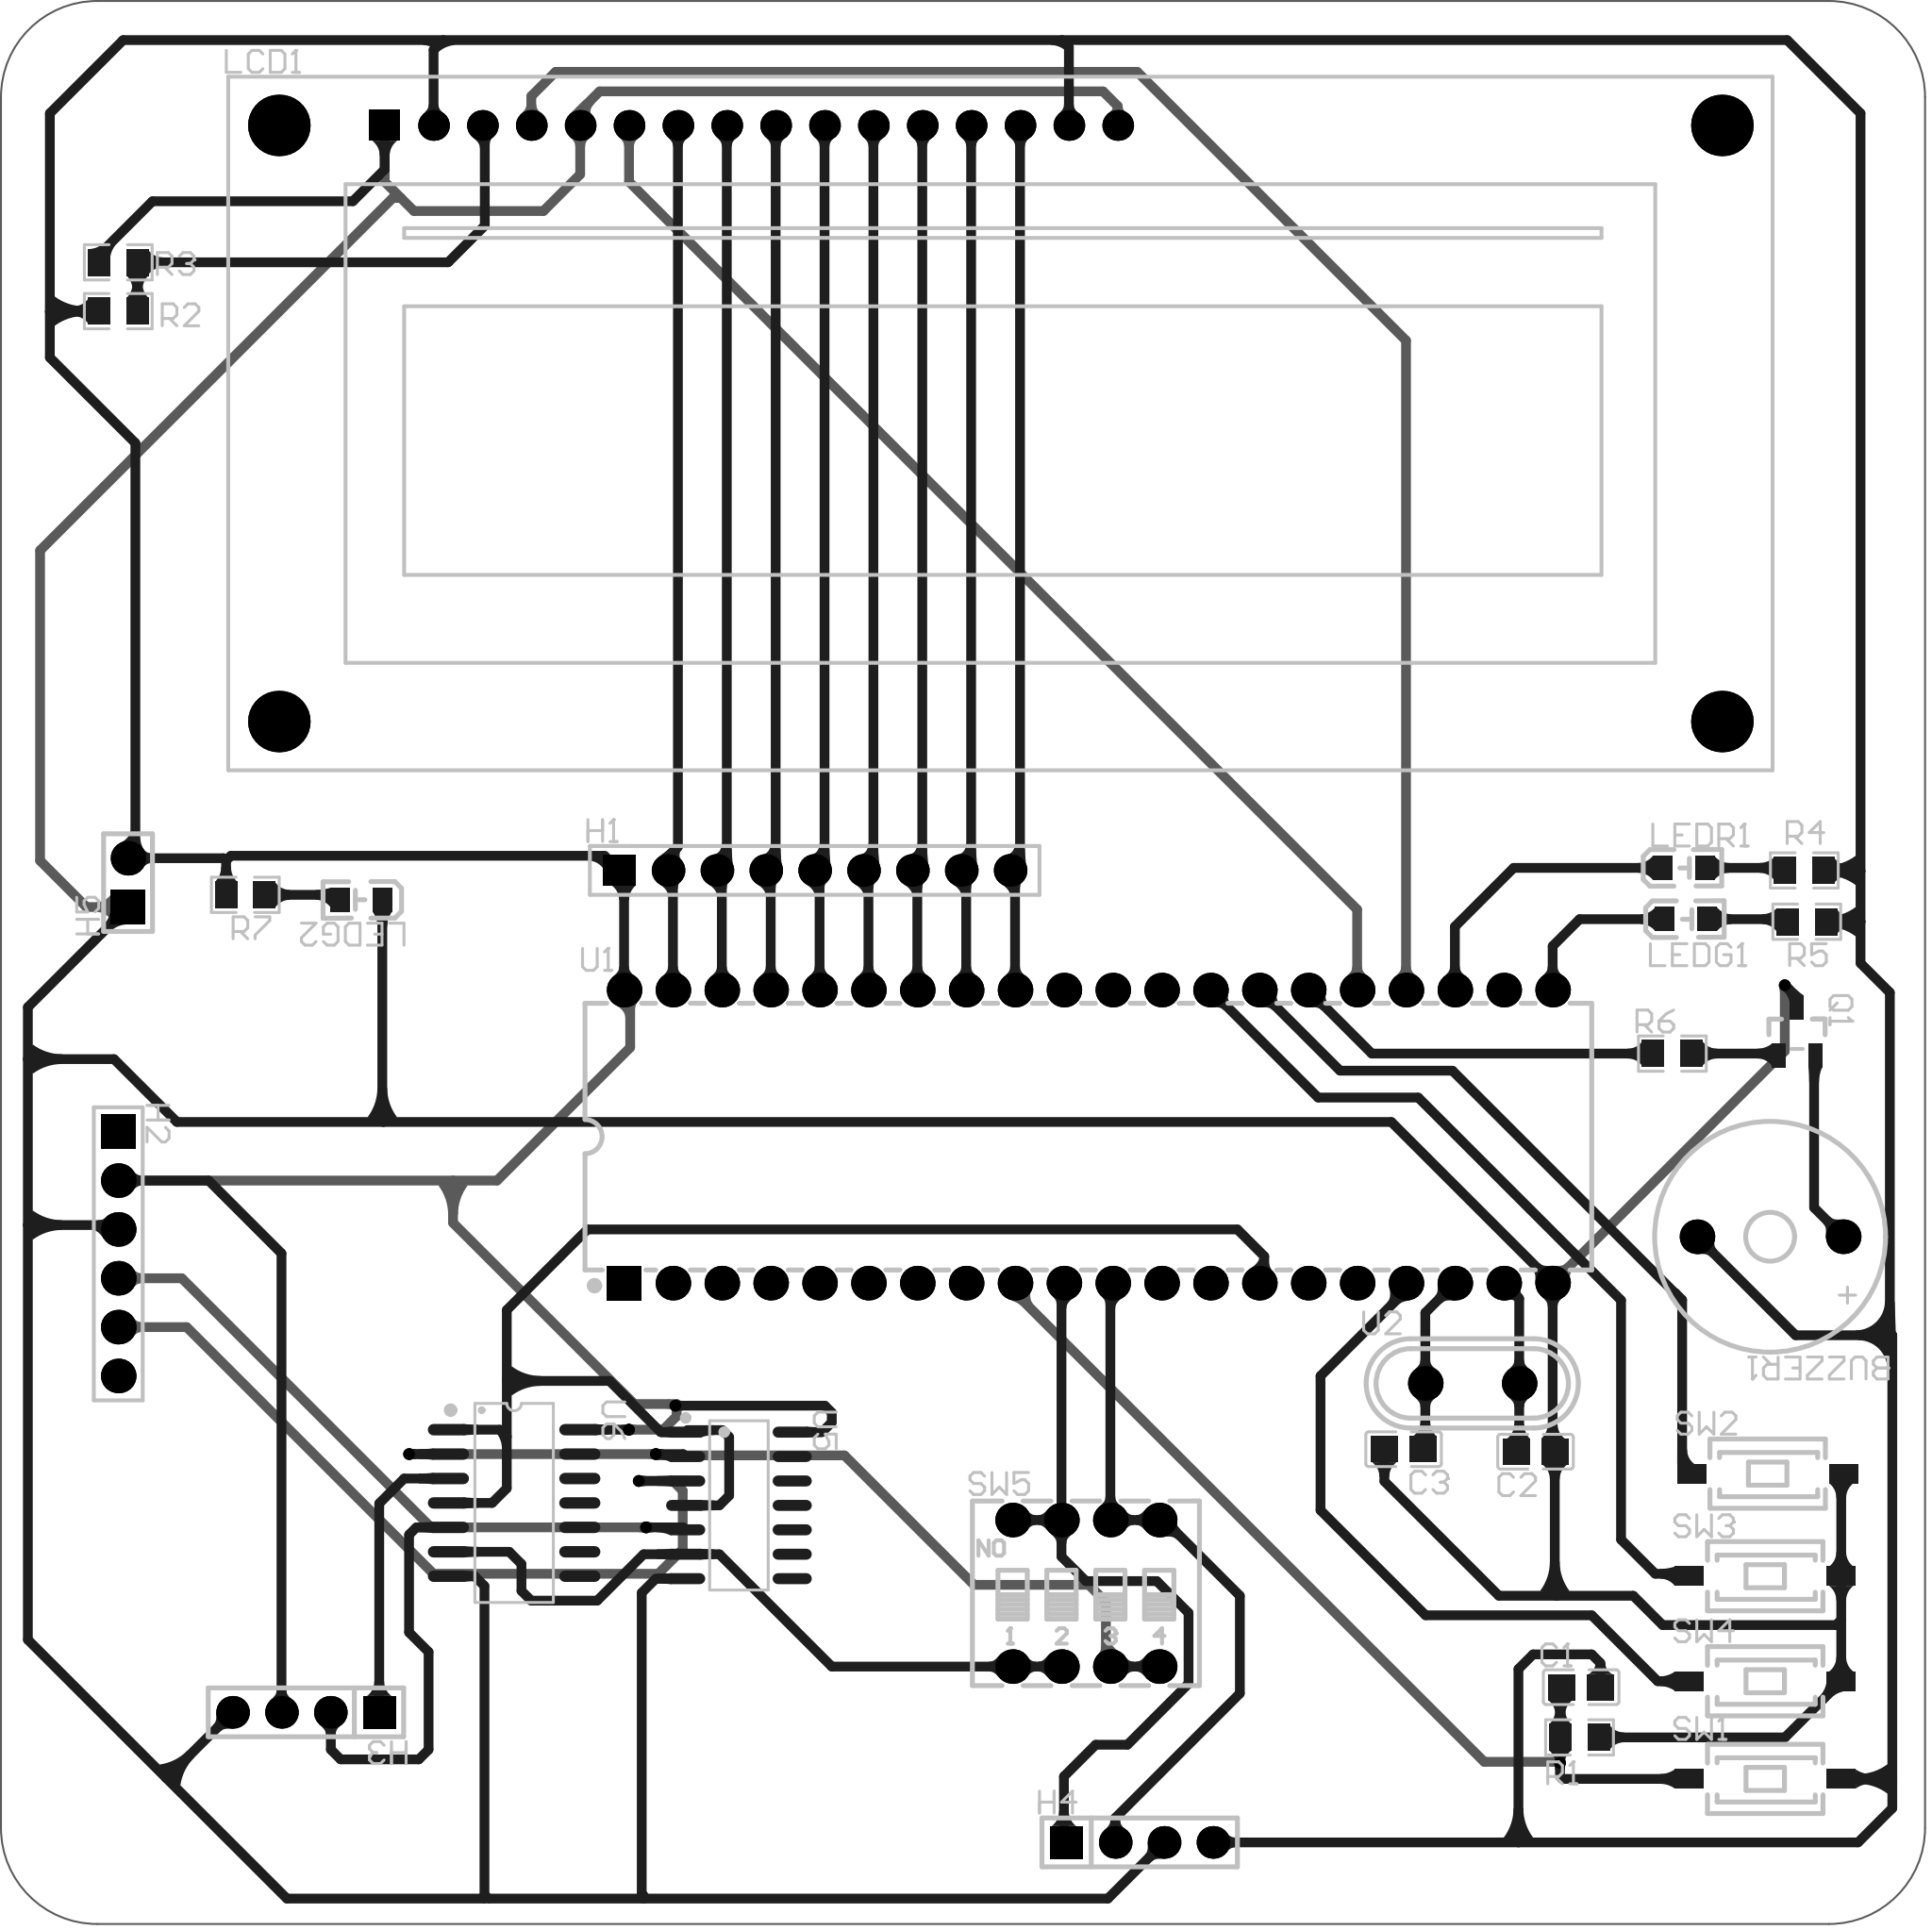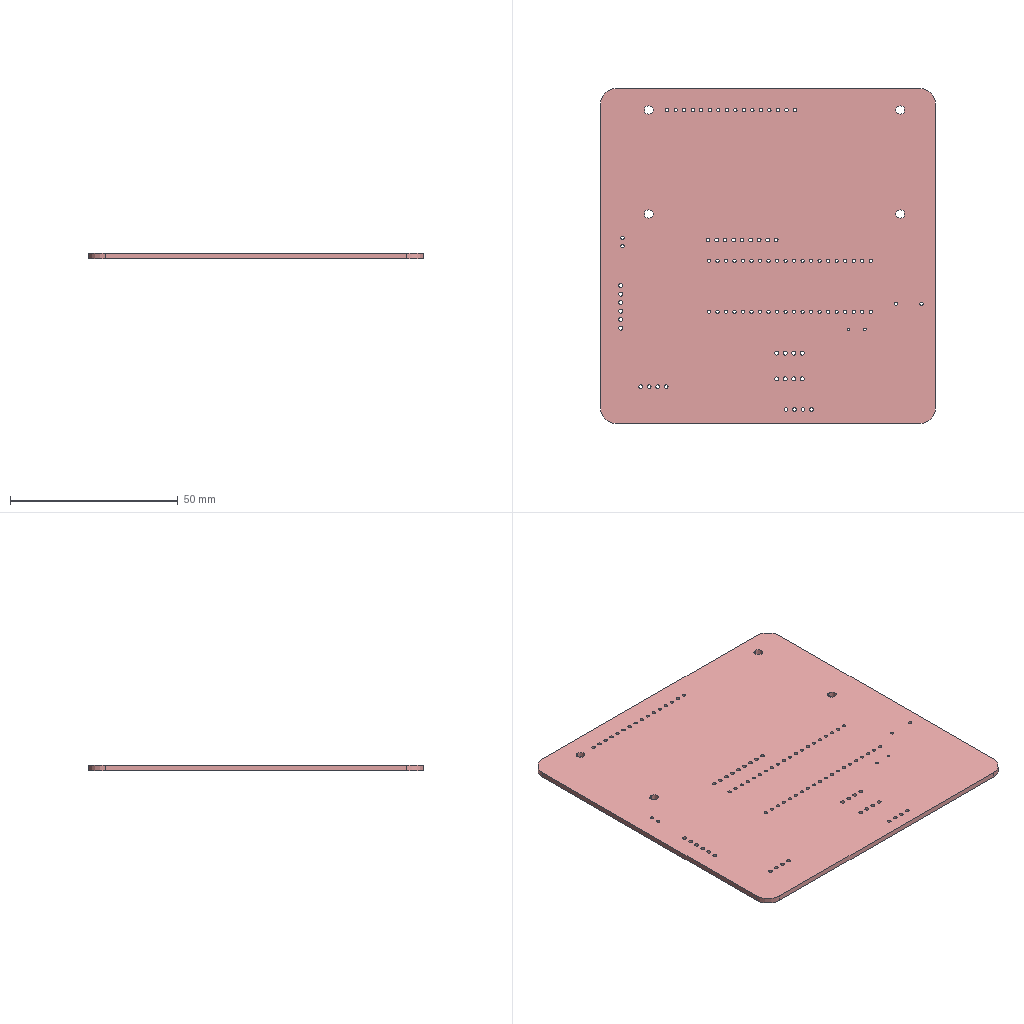Circuit board layout | Altium Designer | box 100 x 100 x 1.6 mm
Layer stack:
# Altium Designer layer stack of  (unit mm; dielectric type: 0 none, 1 core, 2 prepreg, 3 surface material)
index,name,kind,layer,copper_thickness_mm,dielectric_type,dielectric_thickness_mm,dielectric_material,dielectric_constant
0,Top Paste Mask Layer,other,,,,,,
1,Top Silkscreen Layer,other,,,,,,
2,Top Solder Mask Layer,dielectric,,,3,0.01,,3.3
3,Top Layer,copper,Top Layer,0.035,,,,
4,Dielectric1,dielectric,,,3,1.51,FR4,4.5
5,Bottom Layer,copper,Bottom Layer,0.035,,,,
6,Bottom Solder Mask Layer,dielectric,,,3,0.01,,3.3
7,Bottom Silkscreen Layer,other,,,,,,
8,Bottom Paste Mask Layer,other,,,,,,
# drill layer pairs: low layer,high layer
drill_pair,Top Layer,Bottom Layer
Part placement:
Designator,Comment,Layer,Footprint,Center-X(mm),Center-Y(mm),Rotation
BUZZER1,buzzer-12X9,TopLayer,BUZ-TH_BD12.0-P7.60-D0.6-FD,168.148,111.938,180
C1,10uf,TopLayer,C0805,158.327,88.516,0
C2,30pf,TopLayer,C0805,149.098,100.889,0
C3,30pf,TopLayer,C0805,155.956,100.762,180
H1,,TopLayer,HDR-TH_9P-P2.54-V-F-1,118.491,130.988,0
H2,,TopLayer,HDR-TH_6P-P2.54-V-M-1,82.296,111.049,270
H3,,TopLayer,HDR-TH_4P-P2.54-V-M,92.05,87.207,180
H4,,TopLayer,HDR-TH_4P-P2.54-V-M,135.382,80.442,0
LCD1,LMB162ADC,TopLayer,LCD1602,128.143,154.229,0
LEDG1,,TopLayer,LED_0805,163.78,128.453,0
LEDR1,,TopLayer,LED_0805,163.653,131.12,0
Q1,2N3906S-RTK/PS,TopLayer,SOT-23-3_L2.9-W1.3-P1.90-LS2.4-TR,169.545,122.606,270
R1,10K,TopLayer,R0805,158.242,85.903,0
R2,10K,TopLayer,R0805,82.296,160.071,180
R3,1K,TopLayer,R0805,82.296,162.611,0
R4,220,TopLayer,R0805,169.926,130.988,0
R5,220,TopLayer,R0805,170.053,128.321,0
R6,2.2K,TopLayer,R0805,163.068,121.463,0
SW5,DSWB04LHGET,TopLayer,SW-TH_DSWB04LHGET,132.588,93.396,0
U1,STC89C516RD+40I-PDIP40,TopLayer,DIP-40_L52.3-W13.9-P2.54-LS15.2-BL,132.715,117.145,0
U2,11.059MHz,TopLayer,HC-49US_L11.0-W4.6-P4.88,152.667,104.313,0
U5,SN74LS126ADR2,TopLayer,SOIC-14_L8.7-W3.9-P1.27-LS6.0-BL,114.554,97.968,270
U6,DM74LS125ASJ,TopLayer,SOP-14_L10.2-W5.3-P1.27-LS7.8-BL,102.87,98.095,270
LEDG2,,TopLayer,LED_0805,94.919,129.459,180
R7,220,TopLayer,R0805,88.9,129.718,180
H5,,TopLayer,HDR-TH_2P-P2.54-V-M-1,82.804,130.353,90
SW1,Tact switch 3*6*2.5,TopLayer,SW-SMD_L6.0-W3.6-LS8.0,167.894,83.744,0
SW2,Tact switch 3*6*2.5,TopLayer,SW-SMD_L6.0-W3.6-LS8.0,168.021,99.619,0
SW3,Tact switch 3*6*2.5,TopLayer,SW-SMD_L6.0-W3.6-LS8.0,167.894,94.285,0
SW4,Tact switch 3*6*2.5,TopLayer,SW-SMD_L6.0-W3.6-LS8.0,167.894,88.824,0
Pad and via stacks:
# Altium Designer via and pad stacks of  (unit mm). Each distinct definition once, with the count of objects using it.
# via: kind,start_layer,end_layer,hole_mm,diameter_mm,mode(0 simple;1 top-mid-bottom;2 full stack),diameter_per_layer,count,example_net
# pad: kind,layer,hole_mm,hole_type(0 round;1 square;2 slot),plating,top_size,top_shape(1 round;2 rect;3 octagon;9 rounded rect),mid_size,bottom_size,mode,footprint,size_per_layer,count,example
pad,Multi-Layer,1,0,plated,1.8x1.8,1,1.8x1.8,1.8x1.8,0,BUZ-TH_BD12.0-P7.60-D0.6-FD,,2,BUZZER1.2
pad,Multi-Layer,1.1,0,plated,1.7x1.575,2,1.7x1.575,1.7x1.575,0,HDR-TH_9P-P2.54-V-F-1,,1,H1.1
pad,Multi-Layer,1.1,0,plated,1.7x1.7,1,1.7x1.7,1.7x1.7,0,HDR-TH_9P-P2.54-V-F-1,,8,H1.2
pad,Multi-Layer,1.2,0,plated,1.8x1.8,1,1.8x1.8,1.8x1.8,0,HDR-TH_6P-P2.54-V-M-1,,5,H2.6
pad,Multi-Layer,1.2,0,plated,1.8x1.8,2,1.8x1.8,1.8x1.8,0,HDR-TH_6P-P2.54-V-M-1,,1,H2.1
pad,Multi-Layer,1.1,0,plated,1.7x1.7,2,1.7x1.7,1.7x1.7,0,HDR-TH_4P-P2.54-V-M,,2,H3.1
pad,Multi-Layer,1.1,0,plated,1.7x1.7,1,1.7x1.7,1.7x1.7,0,HDR-TH_4P-P2.54-V-M,,6,H3.2
pad,Multi-Layer,1,0,plated,1.6x1.6,1,1.6x1.6,1.6x1.6,0,LCD1602,,15,LCD1.16
pad,Multi-Layer,1,0,plated,1.6x1.6,2,1.6x1.6,1.6x1.6,0,LCD1602,,1,LCD1.1
pad,Multi-Layer,2.5,2,plated,3.2x3.2,1,3.2x3.2,3.2x3.2,0,LCD1602,,4,LCD1.0
pad,Multi-Layer,1.2,0,plated,1.8x1.8,1,1.8x1.8,1.8x1.8,0,SW-TH_DSWB04LHGET,,8,SW5.5
pad,Multi-Layer,1,0,plated,1.8x1.8,1,1.8x1.8,1.8x1.8,0,DIP-40_L52.3-W13.9-P2.54-LS15.2-BL,,39,U1.19
pad,Multi-Layer,1,0,plated,1.8x1.8,2,1.8x1.8,1.8x1.8,0,DIP-40_L52.3-W13.9-P2.54-LS15.2-BL,,1,U1.1
pad,Multi-Layer,0.8,0,plated,1.8x1.8,1,1.8x1.8,1.8x1.8,0,HC-49US_L11.0-W4.6-P4.88,,2,U2.1
pad,Multi-Layer,1,0,plated,1.8x1.8,1,1.8x1.8,1.8x1.8,0,HDR-TH_2P-P2.54-V-M-1,,1,H5.2
pad,Multi-Layer,1,0,plated,1.8x1.8,2,1.8x1.8,1.8x1.8,0,HDR-TH_2P-P2.54-V-M-1,,1,H5.1
pad,Top Layer,0,0,plated,1.41x1.35,2,1.41x1.35,1.41x1.35,0,C0805,,6,C1.2
pad,Top Layer,0,0,plated,1x1.25,2,1x1.25,1x1.25,0,LED_0805,,6,LEDG1.2
pad,Top Layer,0,0,plated,0.7x1.25,2,0.7x1.25,0.7x1.25,0,SOT-23-3_L2.9-W1.3-P1.90-LS2.4-TR,,3,Q1.3
pad,Top Layer,0,0,plated,1.133x1.377,2,1.133x1.377,1.133x1.377,0,R0805,,14,R1.2
pad,Top Layer,0,0,plated,0.574x2.038,1,0.574x2.038,0.574x2.038,0,SOIC-14_L8.7-W3.9-P1.27-LS6.0-BL,,14,U5.1
pad,Top Layer,0,0,plated,0.595x2.143,1,0.595x2.143,0.595x2.143,0,SOP-14_L10.2-W5.3-P1.27-LS7.8-BL,,14,U6.1
pad,Top Layer,0,0,plated,1.5x1,2,1.5x1,1.5x1,0,SW-SMD_L6.0-W3.6-LS8.0,,8,SW1.1
via,Top Layer,Bottom Layer,0.3048,0.6096,0,,7,RX1
via,Top Layer,Bottom Layer,0.3048,0.61,0,,1,$1N2914